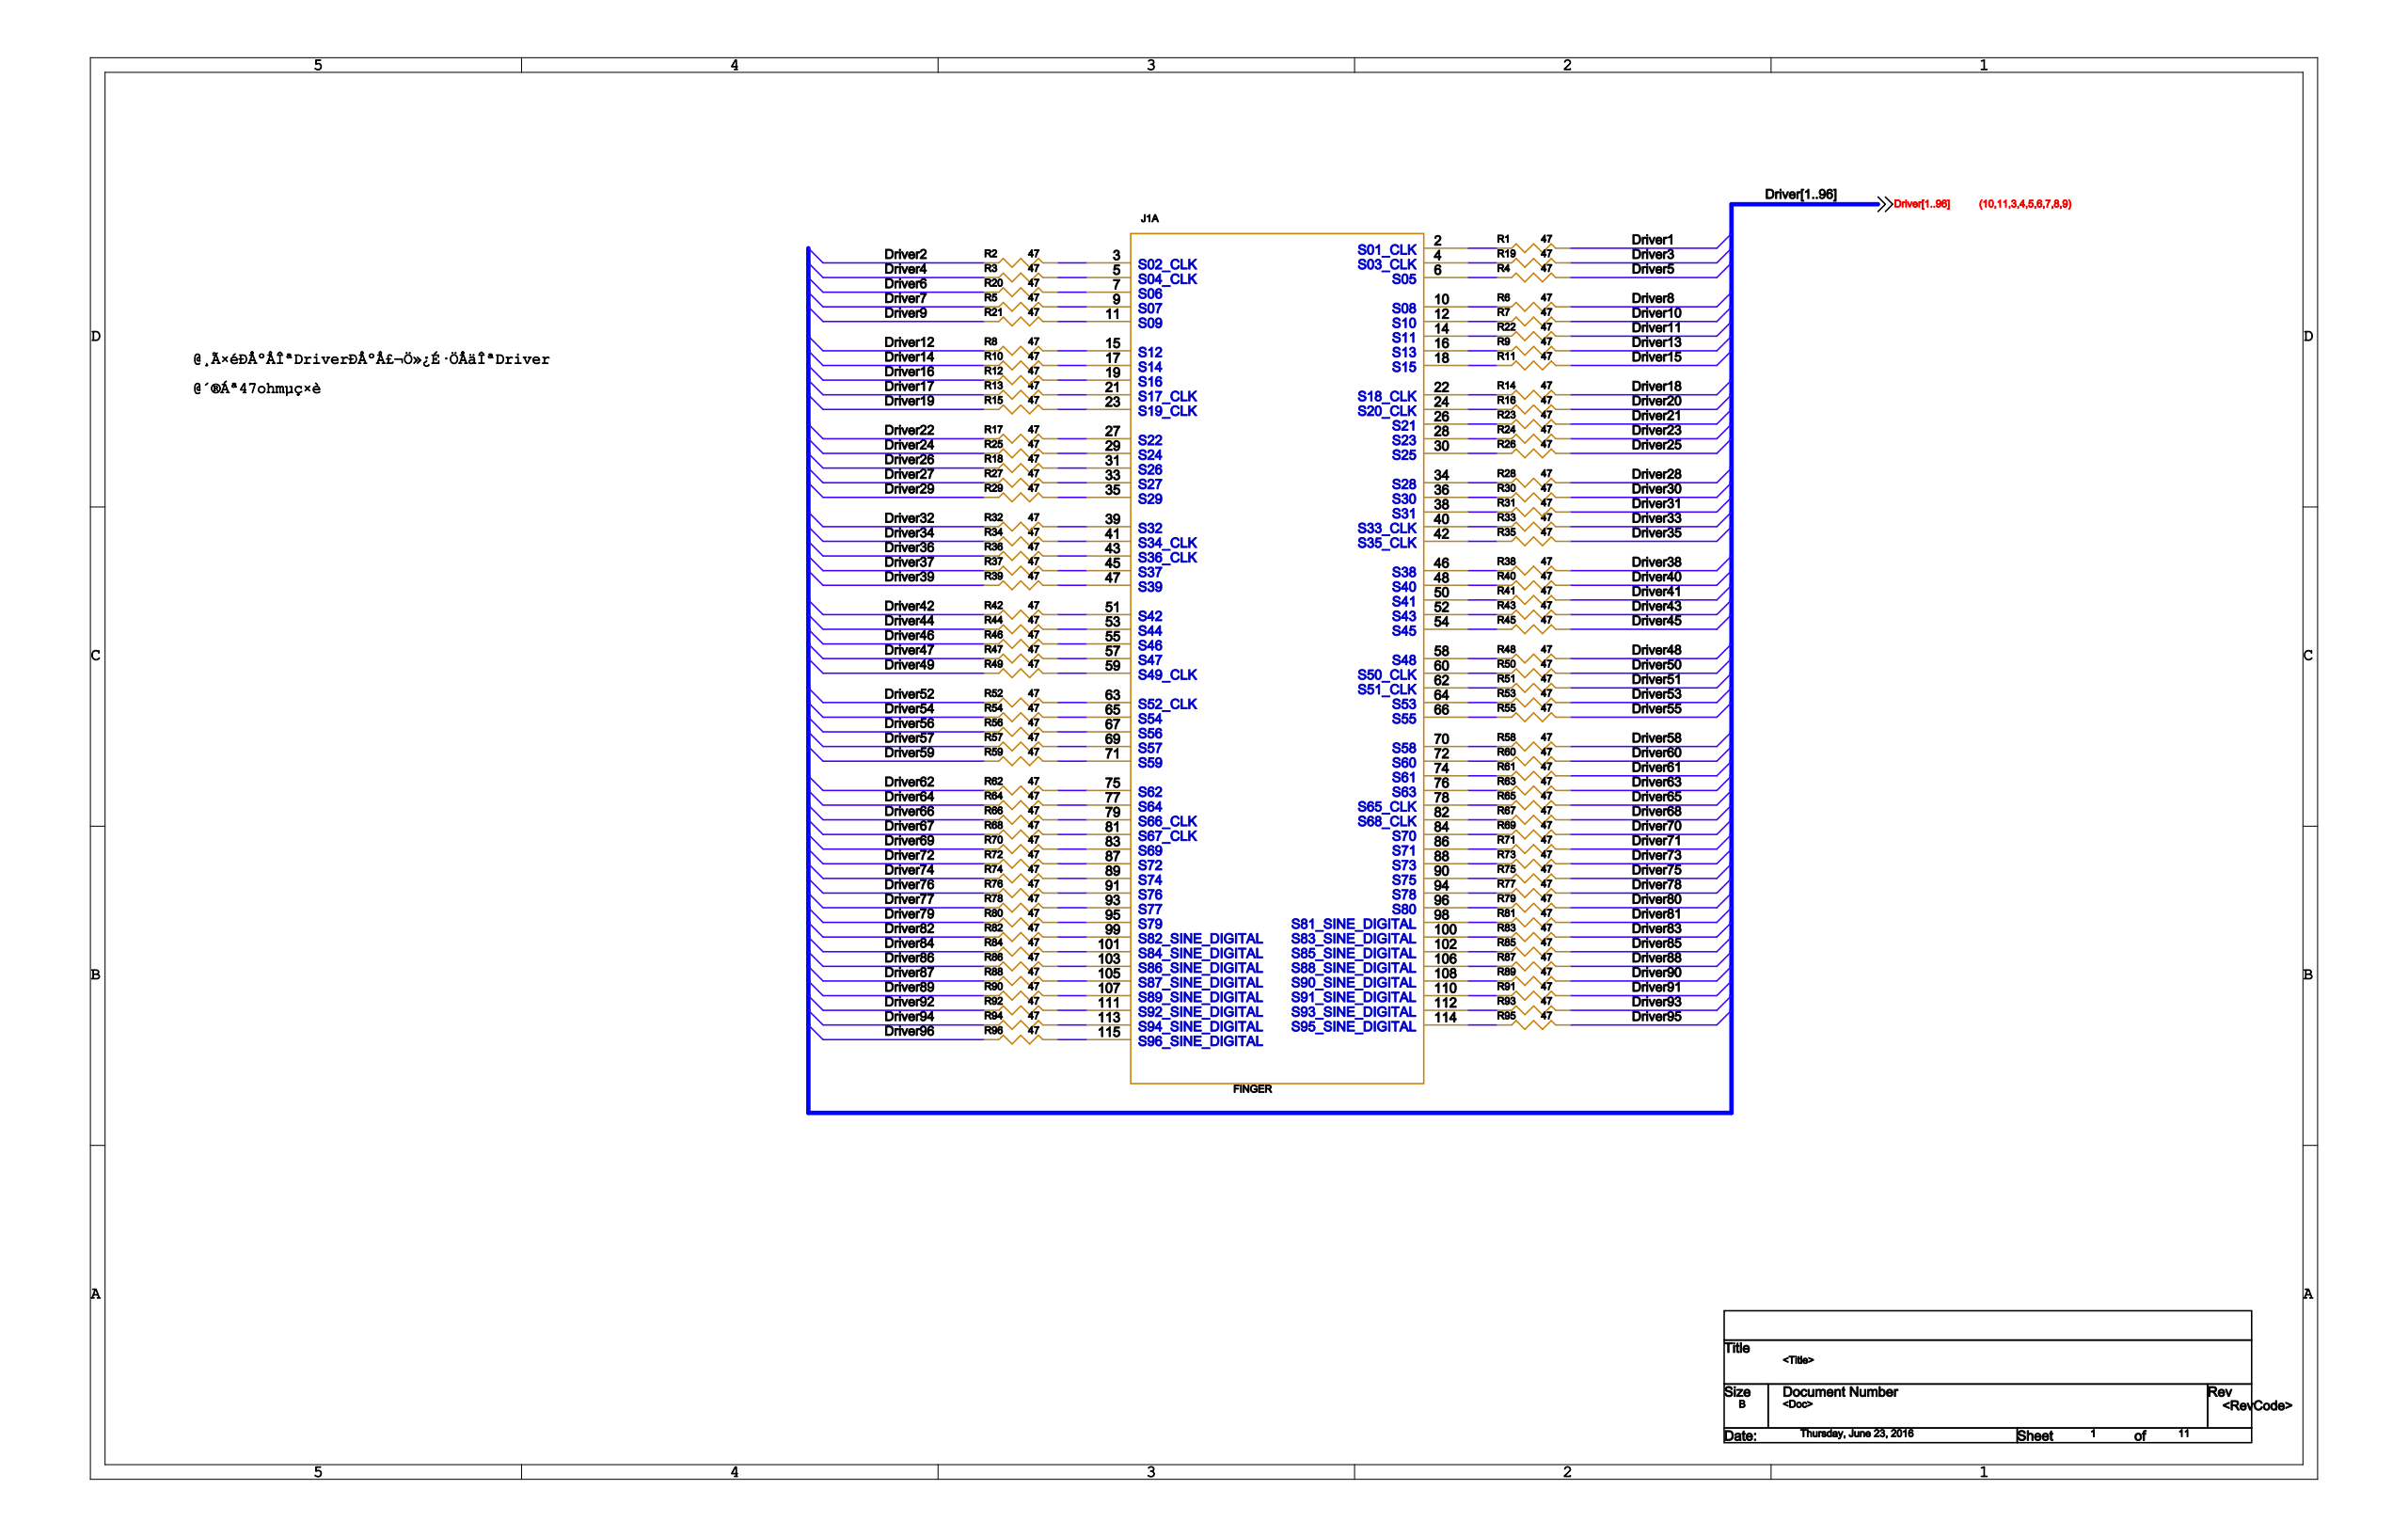Circuit board | Cadence Allegro | 531 parts | 624 nets | one sheet of the schematic
Parts on this sheet (reference | value | footprint):
J1 | FINGER | FINGER
R7 | 47 | RES2-400-100
R25 | 47 | RES2-400-100
R26 | 47 | RES2-400-100
R27 | 47 | RES2-400-100
R28 | 47 | RES2-400-100
R29 | 47 | RES2-400-100
R30 | 47 | RES2-400-100
R31 | 47 | RES2-400-100
R32 | 47 | RES2-400-100
R33 | 47 | RES2-400-100
R34 | 47 | RES2-400-100
R35 | 47 | RES2-400-100
R36 | 47 | RES2-400-100
R37 | 47 | RES2-400-100
R38 | 47 | RES2-400-100
R39 | 47 | RES2-400-100
R40 | 47 | RES2-400-100
R41 | 47 | RES2-400-100
R42 | 47 | RES2-400-100
R43 | 47 | RES2-400-100
R44 | 47 | RES2-400-100
R45 | 47 | RES2-400-100
R46 | 47 | RES2-400-100
R47 | 47 | RES2-400-100
R48 | 47 | RES2-400-100
R49 | 47 | RES2-400-100
R50 | 47 | RES2-400-100
R51 | 47 | RES2-400-100
R52 | 47 | RES2-400-100
R53 | 47 | RES2-400-100
R54 | 47 | RES2-400-100
R55 | 47 | RES2-400-100
R56 | 47 | RES2-400-100
R57 | 47 | RES2-400-100
R58 | 47 | RES2-400-100
R59 | 47 | RES2-400-100
R60 | 47 | RES2-400-100
R61 | 47 | RES2-400-100
R62 | 47 | RES2-400-100
R63 | 47 | RES2-400-100
R64 | 47 | RES2-400-100
R65 | 47 | RES2-400-100
R66 | 47 | RES2-400-100
R67 | 47 | RES2-400-100
R68 | 47 | RES2-400-100
R69 | 47 | RES2-400-100
R70 | 47 | RES2-400-100
R71 | 47 | RES2-400-100
R72 | 47 | RES2-400-100
R73 | 47 | RES2-400-100
R74 | 47 | RES2-400-100
R75 | 47 | RES2-400-100
R76 | 47 | RES2-400-100
R77 | 47 | RES2-400-100
R78 | 47 | RES2-400-100
R79 | 47 | RES2-400-100
R80 | 47 | RES2-400-100
R81 | 47 | RES2-400-100
R82 | 47 | RES2-400-100
R83 | 47 | RES2-400-100
R84 | 47 | RES2-400-100
R85 | 47 | RES2-400-100
R86 | 47 | RES2-400-100
R87 | 47 | RES2-400-100
R88 | 47 | RES2-400-100
R89 | 47 | RES2-400-100
R90 | 47 | RES2-400-100
R91 | 47 | RES2-400-100
R92 | 47 | RES2-400-100
R93 | 47 | RES2-400-100
R94 | 47 | RES2-400-100
R95 | 47 | RES2-400-100
R96 | 47 | RES2-400-100
Nets of these parts (net: part-pin ...):
DRIVER81: R81-2
DRIVER82: R82-1
DRIVER83: R83-2
DRIVER84: R84-1
DRIVER85: R85-2
DRIVER86: R86-1
DRIVER25: R26-2
DRIVER27: R27-1
DRIVER29: R29-1
DRIVER31: R31-2
DRIVER33: R33-2
DRIVER35: R35-2
DRIVER24: R25-1
DRIVER28: R28-2
DRIVER30: R30-2
DRIVER32: R32-1
DRIVER34: R34-1
DRIVER36: R36-1
DRIVER37: R37-1
DRIVER39: R39-1
DRIVER41: R41-2
DRIVER43: R43-2
DRIVER45: R45-2
DRIVER38: R38-2
DRIVER40: R40-2
DRIVER42: R42-1
DRIVER44: R44-1
DRIVER46: R46-1
DRIVER48: R48-2
DRIVER50: R50-2
DRIVER47: R47-1
DRIVER49: R49-1
DRIVER51: R51-2
DRIVER53: R53-2
DRIVER55: R55-2
DRIVER52: R52-1
DRIVER54: R54-1
DRIVER56: R56-1
DRIVER57: R57-1
DRIVER59: R59-1
DRIVER61: R61-2
DRIVER58: R58-2
DRIVER60: R60-2
DRIVER62: R62-1
DRIVER63: R63-2
DRIVER65: R65-2
DRIVER67: R68-1
DRIVER69: R70-1
DRIVER64: R64-1
DRIVER66: R66-1
DRIVER68: R67-2
DRIVER70: R69-2
DRIVER71: R71-2
DRIVER72: R72-1
DRIVER73: R73-2
DRIVER74: R74-1
DRIVER75: R75-2
N6206436: R25-2 J1-29
N6239246: R26-1 J1-30
N6206927: R27-2 J1-33
N6239825: R28-1 J1-34
N6207174: R29-2 J1-35
N6240116: R30-1 J1-36
N6240408: R31-1 J1-38
N6207671: R32-2 J1-39
N6243899: R35-1 J1-42
N6214663: R36-2 J1-43
N6216649: R37-2 J1-45
N6244759: R38-1 J1-46
N6217127: R39-2 J1-47
N6245054: R40-1 J1-48
N6245350: R41-1 J1-50
N6217628: R42-2 J1-51
N6245647: R43-1 J1-52
N6217880: R44-2 J1-53
N6245945: R45-1 J1-54
N6218133: R46-2 J1-55
N6218387: R47-2 J1-57
N6246544: R48-1 J1-58
N6218642: R49-2 J1-59
N6246845: R50-1 J1-60
N6247147: R51-1 J1-62
N6219155: R52-2 J1-63
N6247450: R53-1 J1-64
N6219413: R54-2 J1-65
N6247754: R55-1 J1-66
N6219672: R56-2 J1-67
N6219932: R57-2 J1-69
N6248365: R58-1 J1-70
N6220193: R59-2 J1-71
N6248672: R60-1 J1-72
N6248980: R61-1 J1-74
N6220718: R62-2 J1-75
N6249289: R63-1 J1-76
N6220982: R64-2 J1-77
N6249599: R65-1 J1-78
N6221247: R66-2 J1-79
N6249910: R67-1 J1-82
N6221513: R68-2 J1-81
N6250222: R69-1 J1-84
N6233812: R7-1 J1-12
DRIVER10: R7-2
N6221780: R70-2 J1-83
N6250535: R71-1 J1-86
N6222048: R72-2 J1-87
N6250849: R73-1 J1-88
N6222317: R74-2 J1-89
N6251164: R75-1 J1-90
DRIVER76: R76-1
N6222587: R76-2 J1-91
N6251480: R77-1 J1-94
DRIVER78: R77-2
DRIVER77: R78-1
N6222858: R78-2 J1-93
N6251797: R79-1 J1-96
DRIVER80: R79-2
DRIVER79: R80-1
N6223130: R80-2 J1-95
N6252115: R81-1 J1-98
N6223403: R82-2 J1-99
N6252434: R83-1 J1-100
N6223677: R84-2 J1-101
N6252754: R85-1 J1-102
N6223952: R86-2 J1-103
N6253075: R87-1 J1-106
DRIVER88: R87-2
DRIVER87: R88-1
N6224228: R88-2 J1-105
N6253397: R89-1 J1-108
DRIVER90: R89-2
DRIVER89: R90-1
N6224505: R90-2 J1-107
N6253720: R91-1 J1-110
DRIVER91: R91-2
DRIVER92: R92-1
N6224783: R92-2 J1-111
N6254044: R93-1 J1-112
DRIVER93: R93-2
DRIVER94: R94-1
N6225062: R94-2 J1-113
N6254369: R95-1 J1-114
DRIVER95: R95-2
DRIVER96: R96-1
N6225342: R96-2 J1-115
N4506817: R33-1 J1-40
N4351642: R34-2 J1-41